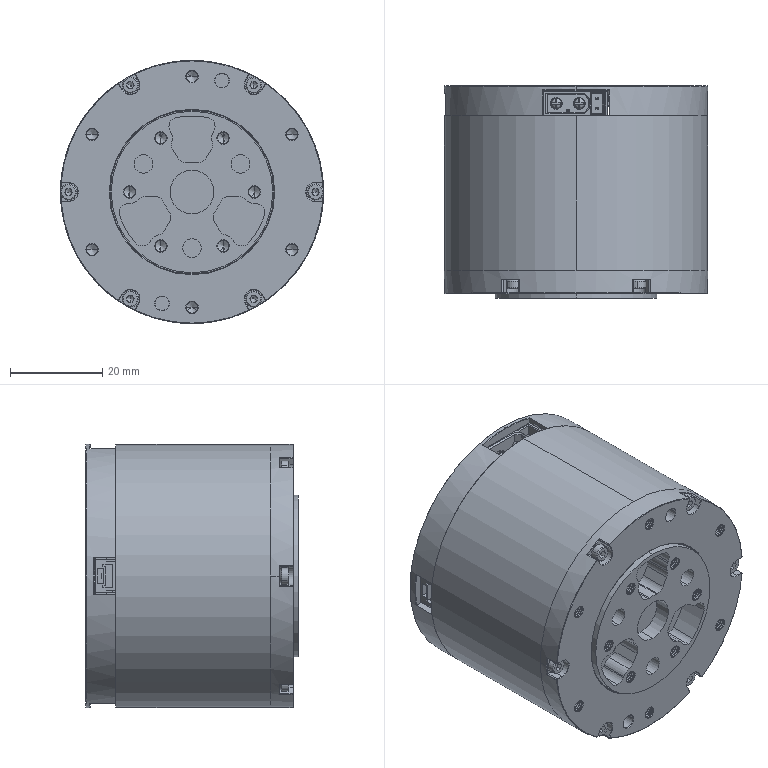Part | SolidWorks | features BaseBody 10 | 10 solids | 2897 faces | box 57 x 46 x 57 mm | volume 102676 mm3 | plane 1144 | cylinder 1051 | spline 379 | cone 297 | torus 26 | commonest cylinder face diameters 2.5 x268 2 x249 0.254 x96 4 x85 0.5 x38 1.6 x28